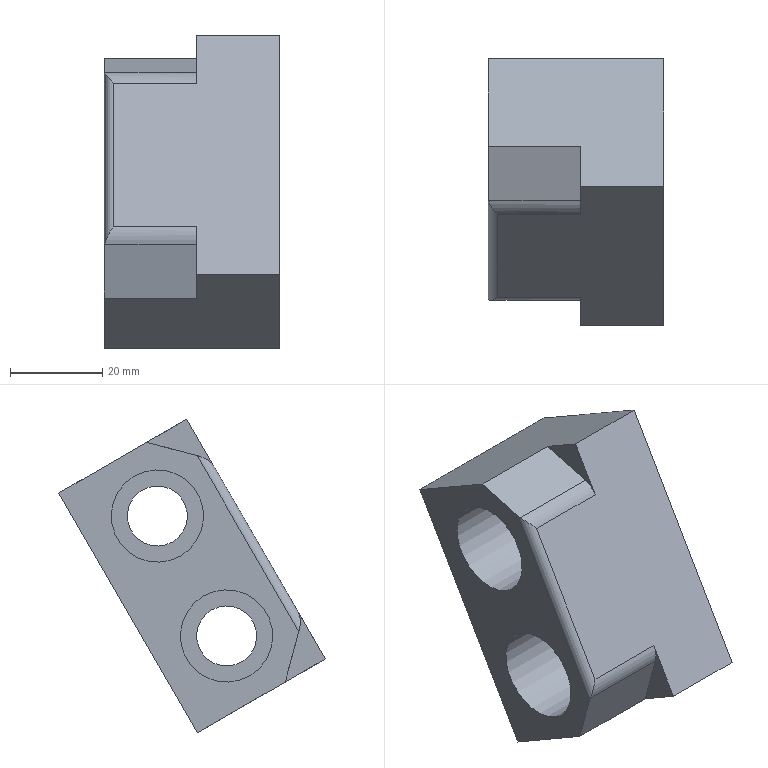Part | NX | features MAIN_BODY 2 | 1 solid | 19 faces | box 38 x 57.713 x 67.962 mm | volume 55374 mm3 | plane 12 | cylinder 7 | commonest cylinder face diameters 10 x2 13 x2 20 x2 4 x1
STEP:
#1=CARTESIAN_POINT('',(-578.,577.963,-16.528));
#2=VERTEX_POINT('',#1);
#3=CARTESIAN_POINT('',(-578.,595.892,14.526));
#4=VERTEX_POINT('',#3);
#5=CARTESIAN_POINT('',(-578.,601.927,24.98));
#6=DIRECTION('',(0.,-0.5,-0.866));
#7=VECTOR('',#6,1000.);
#8=LINE('',#5,#7);
#9=EDGE_CURVE('',#2,#4,#8,.F.);
#10=ORIENTED_EDGE('',*,*,#9,.F.);
#11=CARTESIAN_POINT('',(-560.,577.963,-16.528));
#12=VERTEX_POINT('',#11);
#13=CARTESIAN_POINT('',(-578.,577.963,-16.528));
#14=DIRECTION('',(1.,0.,0.));
#15=VECTOR('',#14,1000.);
#16=LINE('',#13,#15);
#17=EDGE_CURVE('',#12,#2,#16,.F.);
#18=ORIENTED_EDGE('',*,*,#17,.F.);
#19=CARTESIAN_POINT('',(-560.,571.927,-26.982));
#20=VERTEX_POINT('',#19);
#21=CARTESIAN_POINT('',(-560.,601.927,24.98));
#22=DIRECTION('',(0.,-0.5,-0.866));
#23=VECTOR('',#22,1000.);
#24=LINE('',#21,#23);
#25=EDGE_CURVE('',#12,#20,#24,.T.);
#26=ORIENTED_EDGE('',*,*,#25,.T.);
#27=CARTESIAN_POINT('',(-542.,571.927,-26.982));
#28=VERTEX_POINT('',#27);
#29=CARTESIAN_POINT('',(-580.,571.927,-26.982));
#30=DIRECTION('',(1.,0.,0.));
#31=VECTOR('',#30,1000.);
#32=LINE('',#29,#31);
#33=EDGE_CURVE('',#20,#28,#32,.T.);
#34=ORIENTED_EDGE('',*,*,#33,.T.);
#35=CARTESIAN_POINT('',(-542.,601.927,24.98));
#36=VERTEX_POINT('',#35);
#37=CARTESIAN_POINT('',(-542.,601.927,24.98));
#38=DIRECTION('',(0.,-0.5,-0.866));
#39=VECTOR('',#38,1000.);
#40=LINE('',#37,#39);
#41=EDGE_CURVE('',#36,#28,#40,.T.);
#42=ORIENTED_EDGE('',*,*,#41,.F.);
#43=CARTESIAN_POINT('',(-560.,601.927,24.98));
#44=VERTEX_POINT('',#43);
#45=CARTESIAN_POINT('',(-580.,601.927,24.98));
#46=DIRECTION('',(1.,0.,0.));
#47=VECTOR('',#46,1000.);
#48=LINE('',#45,#47);
#49=EDGE_CURVE('',#44,#36,#48,.T.);
#50=ORIENTED_EDGE('',*,*,#49,.F.);
#51=CARTESIAN_POINT('',(-560.,595.892,14.526));
#52=VERTEX_POINT('',#51);
#53=CARTESIAN_POINT('',(-560.,601.927,24.98));
#54=DIRECTION('',(0.,-0.5,-0.866));
#55=VECTOR('',#54,1000.);
#56=LINE('',#53,#55);
#57=EDGE_CURVE('',#44,#52,#56,.T.);
#58=ORIENTED_EDGE('',*,*,#57,.T.);
#59=CARTESIAN_POINT('',(-560.,595.892,14.526));
#60=DIRECTION('',(1.,0.,0.));
#61=VECTOR('',#60,1000.);
#62=LINE('',#59,#61);
#63=EDGE_CURVE('',#4,#52,#62,.T.);
#64=ORIENTED_EDGE('',*,*,#63,.F.);
#65=EDGE_LOOP('',(#10,#18,#26,#34,#42,#50,#58,#64));
#66=FACE_BOUND('',#65,.T.);
#67=CARTESIAN_POINT('',(-580.,601.927,24.98));
#68=DIRECTION('',(0.,0.866,-0.5));
#69=DIRECTION('',(0.,-0.5,-0.866));
#70=AXIS2_PLACEMENT_3D('',#67,#68,#69);
#71=PLANE('',#70);
#72=ADVANCED_FACE('',(#66),#71,.F.);
#73=CARTESIAN_POINT('',(-580.,613.284,12.649));
#74=VERTEX_POINT('',#73);
#75=CARTESIAN_POINT('',(-580.,608.284,3.989));
#76=DIRECTION('',(-1.,0.,0.));
#77=DIRECTION('',(0.,0.5,0.866));
#78=AXIS2_PLACEMENT_3D('',#75,#76,#77);
#79=CIRCLE('',#78,10.);
#80=EDGE_CURVE('',#74,#74,#79,.T.);
#81=ORIENTED_EDGE('',*,*,#80,.F.);
#82=EDGE_LOOP('',(#81));
#83=FACE_BOUND('',#82,.T.);
#84=CARTESIAN_POINT('',(-580.,598.284,-13.331));
#85=VERTEX_POINT('',#84);
#86=CARTESIAN_POINT('',(-580.,593.284,-21.992));
#87=DIRECTION('',(-1.,0.,0.));
#88=DIRECTION('',(0.,0.5,0.866));
#89=AXIS2_PLACEMENT_3D('',#86,#87,#88);
#90=CIRCLE('',#89,10.);
#91=EDGE_CURVE('',#85,#85,#90,.T.);
#92=ORIENTED_EDGE('',*,*,#91,.F.);
#93=EDGE_LOOP('',(#92));
#94=FACE_BOUND('',#93,.T.);
#95=CARTESIAN_POINT('',(-580.,599.659,17.051));
#96=VERTEX_POINT('',#95);
#97=CARTESIAN_POINT('',(-580.,610.588,19.98));
#98=VERTEX_POINT('',#97);
#99=CARTESIAN_POINT('',(-580.,596.927,16.319));
#100=DIRECTION('',(0.,0.9659,0.2588));
#101=VECTOR('',#100,1000.);
#102=LINE('',#99,#101);
#103=EDGE_CURVE('',#96,#98,#102,.T.);
#104=ORIENTED_EDGE('',*,*,#103,.T.);
#105=CARTESIAN_POINT('',(-580.,629.64,8.98));
#106=VERTEX_POINT('',#105);
#107=CARTESIAN_POINT('',(-580.,629.64,8.98));
#108=DIRECTION('',(0.,-0.866,0.5));
#109=VECTOR('',#108,1000.);
#110=LINE('',#107,#109);
#111=EDGE_CURVE('',#106,#98,#110,.T.);
#112=ORIENTED_EDGE('',*,*,#111,.F.);
#113=CARTESIAN_POINT('',(-580.,599.64,-42.982));
#114=VERTEX_POINT('',#113);
#115=CARTESIAN_POINT('',(-580.,599.64,-42.982));
#116=DIRECTION('',(0.,0.5,0.866));
#117=VECTOR('',#116,1000.);
#118=LINE('',#115,#117);
#119=EDGE_CURVE('',#114,#106,#118,.T.);
#120=ORIENTED_EDGE('',*,*,#119,.F.);
#121=CARTESIAN_POINT('',(-580.,580.588,-31.982));
#122=VERTEX_POINT('',#121);
#123=CARTESIAN_POINT('',(-580.,571.927,-26.982));
#124=DIRECTION('',(0.,0.866,-0.5));
#125=VECTOR('',#124,1000.);
#126=LINE('',#123,#125);
#127=EDGE_CURVE('',#122,#114,#126,.T.);
#128=ORIENTED_EDGE('',*,*,#127,.F.);
#129=CARTESIAN_POINT('',(-580.,577.659,-21.054));
#130=VERTEX_POINT('',#129);
#131=CARTESIAN_POINT('',(-580.,580.588,-31.982));
#132=DIRECTION('',(0.,-0.2588,0.9659));
#133=VECTOR('',#132,1000.);
#134=LINE('',#131,#133);
#135=EDGE_CURVE('',#122,#130,#134,.T.);
#136=ORIENTED_EDGE('',*,*,#135,.T.);
#137=CARTESIAN_POINT('',(-580.,573.659,-27.982));
#138=DIRECTION('',(0.,-0.5,-0.866));
#139=VECTOR('',#138,1000.);
#140=LINE('',#137,#139);
#141=EDGE_CURVE('',#96,#130,#140,.T.);
#142=ORIENTED_EDGE('',*,*,#141,.F.);
#143=EDGE_LOOP('',(#104,#112,#120,#128,#136,#142));
#144=FACE_BOUND('',#143,.T.);
#145=CARTESIAN_POINT('',(-580.,599.64,-42.982));
#146=DIRECTION('',(1.,0.,0.));
#147=DIRECTION('',(0.,0.5,0.866));
#148=AXIS2_PLACEMENT_3D('',#145,#146,#147);
#149=PLANE('',#148);
#150=ADVANCED_FACE('',(#83,#94,#144),#149,.F.);
#151=CARTESIAN_POINT('',(-560.,580.588,-31.982));
#152=VERTEX_POINT('',#151);
#153=CARTESIAN_POINT('',(-560.,571.927,-26.982));
#154=DIRECTION('',(0.,0.866,-0.5));
#155=VECTOR('',#154,1000.);
#156=LINE('',#153,#155);
#157=EDGE_CURVE('',#20,#152,#156,.T.);
#158=ORIENTED_EDGE('',*,*,#157,.T.);
#159=CARTESIAN_POINT('',(-580.,580.588,-31.982));
#160=DIRECTION('',(1.,0.,0.));
#161=VECTOR('',#160,1000.);
#162=LINE('',#159,#161);
#163=EDGE_CURVE('',#122,#152,#162,.T.);
#164=ORIENTED_EDGE('',*,*,#163,.F.);
#165=ORIENTED_EDGE('',*,*,#127,.T.);
#166=CARTESIAN_POINT('',(-542.,599.64,-42.982));
#167=VERTEX_POINT('',#166);
#168=CARTESIAN_POINT('',(-580.,599.64,-42.982));
#169=DIRECTION('',(1.,0.,0.));
#170=VECTOR('',#169,1000.);
#171=LINE('',#168,#170);
#172=EDGE_CURVE('',#114,#167,#171,.T.);
#173=ORIENTED_EDGE('',*,*,#172,.T.);
#174=CARTESIAN_POINT('',(-542.,571.927,-26.982));
#175=DIRECTION('',(0.,0.866,-0.5));
#176=VECTOR('',#175,1000.);
#177=LINE('',#174,#176);
#178=EDGE_CURVE('',#28,#167,#177,.T.);
#179=ORIENTED_EDGE('',*,*,#178,.F.);
#180=ORIENTED_EDGE('',*,*,#33,.F.);
#181=EDGE_LOOP('',(#158,#164,#165,#173,#179,#180));
#182=FACE_BOUND('',#181,.T.);
#183=CARTESIAN_POINT('',(-580.,571.927,-26.982));
#184=DIRECTION('',(0.,0.5,0.866));
#185=DIRECTION('',(-1.,0.,0.));
#186=AXIS2_PLACEMENT_3D('',#183,#184,#185);
#187=PLANE('',#186);
#188=ADVANCED_FACE('',(#182),#187,.F.);
#189=CARTESIAN_POINT('',(-560.,610.588,19.98));
#190=VERTEX_POINT('',#189);
#191=CARTESIAN_POINT('',(-560.,629.64,8.98));
#192=DIRECTION('',(0.,-0.866,0.5));
#193=VECTOR('',#192,1000.);
#194=LINE('',#191,#193);
#195=EDGE_CURVE('',#190,#44,#194,.T.);
#196=ORIENTED_EDGE('',*,*,#195,.T.);
#197=ORIENTED_EDGE('',*,*,#49,.T.);
#198=CARTESIAN_POINT('',(-542.,629.64,8.98));
#199=VERTEX_POINT('',#198);
#200=CARTESIAN_POINT('',(-542.,629.64,8.98));
#201=DIRECTION('',(0.,-0.866,0.5));
#202=VECTOR('',#201,1000.);
#203=LINE('',#200,#202);
#204=EDGE_CURVE('',#199,#36,#203,.T.);
#205=ORIENTED_EDGE('',*,*,#204,.F.);
#206=CARTESIAN_POINT('',(-580.,629.64,8.98));
#207=DIRECTION('',(1.,0.,0.));
#208=VECTOR('',#207,1000.);
#209=LINE('',#206,#208);
#210=EDGE_CURVE('',#106,#199,#209,.T.);
#211=ORIENTED_EDGE('',*,*,#210,.F.);
#212=ORIENTED_EDGE('',*,*,#111,.T.);
#213=CARTESIAN_POINT('',(-580.,610.588,19.98));
#214=DIRECTION('',(1.,0.,0.));
#215=VECTOR('',#214,1000.);
#216=LINE('',#213,#215);
#217=EDGE_CURVE('',#98,#190,#216,.T.);
#218=ORIENTED_EDGE('',*,*,#217,.T.);
#219=EDGE_LOOP('',(#196,#197,#205,#211,#212,#218));
#220=FACE_BOUND('',#219,.T.);
#221=CARTESIAN_POINT('',(-580.,629.64,8.98));
#222=DIRECTION('',(0.,-0.5,-0.866));
#223=DIRECTION('',(0.,-0.866,0.5));
#224=AXIS2_PLACEMENT_3D('',#221,#222,#223);
#225=PLANE('',#224);
#226=ADVANCED_FACE('',(#220),#225,.F.);
#227=CARTESIAN_POINT('',(-542.,599.64,-42.982));
#228=DIRECTION('',(0.,0.5,0.866));
#229=VECTOR('',#228,1000.);
#230=LINE('',#227,#229);
#231=EDGE_CURVE('',#167,#199,#230,.T.);
#232=ORIENTED_EDGE('',*,*,#231,.F.);
#233=ORIENTED_EDGE('',*,*,#172,.F.);
#234=ORIENTED_EDGE('',*,*,#119,.T.);
#235=ORIENTED_EDGE('',*,*,#210,.T.);
#236=EDGE_LOOP('',(#232,#233,#234,#235));
#237=FACE_BOUND('',#236,.T.);
#238=CARTESIAN_POINT('',(-580.,599.64,-42.982));
#239=DIRECTION('',(0.,-0.866,0.5));
#240=DIRECTION('',(-1.,0.,0.));
#241=AXIS2_PLACEMENT_3D('',#238,#239,#240);
#242=PLANE('',#241);
#243=ADVANCED_FACE('',(#237),#242,.F.);
#244=CARTESIAN_POINT('',(-565.,611.534,9.618));
#245=VERTEX_POINT('',#244);
#246=CARTESIAN_POINT('',(-565.,608.284,3.989));
#247=DIRECTION('',(-1.,0.,0.));
#248=DIRECTION('',(0.,0.5,0.866));
#249=AXIS2_PLACEMENT_3D('',#246,#247,#248);
#250=CIRCLE('',#249,6.5);
#251=EDGE_CURVE('',#245,#245,#250,.F.);
#252=ORIENTED_EDGE('',*,*,#251,.F.);
#253=EDGE_LOOP('',(#252));
#254=FACE_BOUND('',#253,.T.);
#255=CARTESIAN_POINT('',(-542.,611.534,9.618));
#256=VERTEX_POINT('',#255);
#257=CARTESIAN_POINT('',(-542.,608.284,3.989));
#258=DIRECTION('',(-1.,0.,0.));
#259=DIRECTION('',(0.,0.5,0.866));
#260=AXIS2_PLACEMENT_3D('',#257,#258,#259);
#261=CIRCLE('',#260,6.5);
#262=EDGE_CURVE('',#256,#256,#261,.T.);
#263=ORIENTED_EDGE('',*,*,#262,.F.);
#264=EDGE_LOOP('',(#263));
#265=FACE_BOUND('',#264,.T.);
#266=CARTESIAN_POINT('',(-580.,608.284,3.989));
#267=DIRECTION('',(1.,0.,0.));
#268=DIRECTION('',(0.,0.5,0.866));
#269=AXIS2_PLACEMENT_3D('',#266,#267,#268);
#270=CYLINDRICAL_SURFACE('',#269,6.5);
#271=ADVANCED_FACE('',(#254,#265),#270,.F.);
#272=CARTESIAN_POINT('',(-565.,596.534,-16.362));
#273=VERTEX_POINT('',#272);
#274=CARTESIAN_POINT('',(-565.,593.284,-21.992));
#275=DIRECTION('',(-1.,0.,0.));
#276=DIRECTION('',(0.,0.5,0.866));
#277=AXIS2_PLACEMENT_3D('',#274,#275,#276);
#278=CIRCLE('',#277,6.5);
#279=EDGE_CURVE('',#273,#273,#278,.F.);
#280=ORIENTED_EDGE('',*,*,#279,.F.);
#281=EDGE_LOOP('',(#280));
#282=FACE_BOUND('',#281,.T.);
#283=CARTESIAN_POINT('',(-542.,596.534,-16.362));
#284=VERTEX_POINT('',#283);
#285=CARTESIAN_POINT('',(-542.,593.284,-21.992));
#286=DIRECTION('',(-1.,0.,0.));
#287=DIRECTION('',(0.,0.5,0.866));
#288=AXIS2_PLACEMENT_3D('',#285,#286,#287);
#289=CIRCLE('',#288,6.5);
#290=EDGE_CURVE('',#284,#284,#289,.T.);
#291=ORIENTED_EDGE('',*,*,#290,.F.);
#292=EDGE_LOOP('',(#291));
#293=FACE_BOUND('',#292,.T.);
#294=CARTESIAN_POINT('',(-580.,593.284,-21.992));
#295=DIRECTION('',(1.,0.,0.));
#296=DIRECTION('',(0.,0.5,0.866));
#297=AXIS2_PLACEMENT_3D('',#294,#295,#296);
#298=CYLINDRICAL_SURFACE('',#297,6.5);
#299=ADVANCED_FACE('',(#282,#293),#298,.F.);
#300=ORIENTED_EDGE('',*,*,#262,.T.);
#301=EDGE_LOOP('',(#300));
#302=FACE_BOUND('',#301,.T.);
#303=ORIENTED_EDGE('',*,*,#231,.T.);
#304=ORIENTED_EDGE('',*,*,#204,.T.);
#305=ORIENTED_EDGE('',*,*,#41,.T.);
#306=ORIENTED_EDGE('',*,*,#178,.T.);
#307=EDGE_LOOP('',(#303,#304,#305,#306));
#308=FACE_BOUND('',#307,.T.);
#309=ORIENTED_EDGE('',*,*,#290,.T.);
#310=EDGE_LOOP('',(#309));
#311=FACE_BOUND('',#310,.T.);
#312=CARTESIAN_POINT('',(-542.,599.64,-42.982));
#313=DIRECTION('',(1.,0.,0.));
#314=DIRECTION('',(0.,0.5,0.866));
#315=AXIS2_PLACEMENT_3D('',#312,#313,#314);
#316=PLANE('',#315);
#317=ADVANCED_FACE('',(#302,#308,#311),#316,.T.);
#318=CARTESIAN_POINT('',(-565.,598.284,-13.331));
#319=VERTEX_POINT('',#318);
#320=CARTESIAN_POINT('',(-565.,593.284,-21.992));
#321=DIRECTION('',(-1.,0.,0.));
#322=DIRECTION('',(0.,0.5,0.866));
#323=AXIS2_PLACEMENT_3D('',#320,#321,#322);
#324=CIRCLE('',#323,10.);
#325=EDGE_CURVE('',#319,#319,#324,.T.);
#326=ORIENTED_EDGE('',*,*,#325,.T.);
#327=EDGE_LOOP('',(#326));
#328=FACE_BOUND('',#327,.T.);
#329=ORIENTED_EDGE('',*,*,#279,.T.);
#330=EDGE_LOOP('',(#329));
#331=FACE_BOUND('',#330,.T.);
#332=CARTESIAN_POINT('',(-565.,593.284,-21.992));
#333=DIRECTION('',(1.,0.,0.));
#334=DIRECTION('',(0.,0.5,0.866));
#335=AXIS2_PLACEMENT_3D('',#332,#333,#334);
#336=PLANE('',#335);
#337=ADVANCED_FACE('',(#328,#331),#336,.F.);
#338=ORIENTED_EDGE('',*,*,#91,.T.);
#339=EDGE_LOOP('',(#338));
#340=FACE_BOUND('',#339,.T.);
#341=ORIENTED_EDGE('',*,*,#325,.F.);
#342=EDGE_LOOP('',(#341));
#343=FACE_BOUND('',#342,.T.);
#344=CARTESIAN_POINT('',(-580.,593.284,-21.992));
#345=DIRECTION('',(1.,0.,0.));
#346=DIRECTION('',(0.,0.5,0.866));
#347=AXIS2_PLACEMENT_3D('',#344,#345,#346);
#348=CYLINDRICAL_SURFACE('',#347,10.);
#349=ADVANCED_FACE('',(#340,#343),#348,.F.);
#350=CARTESIAN_POINT('',(-565.,613.284,12.649));
#351=VERTEX_POINT('',#350);
#352=CARTESIAN_POINT('',(-565.,608.284,3.989));
#353=DIRECTION('',(-1.,0.,0.));
#354=DIRECTION('',(0.,0.5,0.866));
#355=AXIS2_PLACEMENT_3D('',#352,#353,#354);
#356=CIRCLE('',#355,10.);
#357=EDGE_CURVE('',#351,#351,#356,.T.);
#358=ORIENTED_EDGE('',*,*,#357,.T.);
#359=EDGE_LOOP('',(#358));
#360=FACE_BOUND('',#359,.T.);
#361=ORIENTED_EDGE('',*,*,#251,.T.);
#362=EDGE_LOOP('',(#361));
#363=FACE_BOUND('',#362,.T.);
#364=CARTESIAN_POINT('',(-565.,608.284,3.989));
#365=DIRECTION('',(1.,0.,0.));
#366=DIRECTION('',(0.,0.5,0.866));
#367=AXIS2_PLACEMENT_3D('',#364,#365,#366);
#368=PLANE('',#367);
#369=ADVANCED_FACE('',(#360,#363),#368,.F.);
#370=ORIENTED_EDGE('',*,*,#80,.T.);
#371=EDGE_LOOP('',(#370));
#372=FACE_BOUND('',#371,.T.);
#373=ORIENTED_EDGE('',*,*,#357,.F.);
#374=EDGE_LOOP('',(#373));
#375=FACE_BOUND('',#374,.T.);
#376=CARTESIAN_POINT('',(-580.,608.284,3.989));
#377=DIRECTION('',(1.,0.,0.));
#378=DIRECTION('',(0.,0.5,0.866));
#379=AXIS2_PLACEMENT_3D('',#376,#377,#378);
#380=CYLINDRICAL_SURFACE('',#379,10.);
#381=ADVANCED_FACE('',(#372,#375),#380,.F.);
#382=ORIENTED_EDGE('',*,*,#195,.F.);
#383=CARTESIAN_POINT('',(-560.,598.928,16.855));
#384=VERTEX_POINT('',#383);
#385=CARTESIAN_POINT('',(-560.,596.927,16.319));
#386=DIRECTION('',(0.,0.9659,0.2588));
#387=VECTOR('',#386,1000.);
#388=LINE('',#385,#387);
#389=EDGE_CURVE('',#384,#190,#388,.T.);
#390=ORIENTED_EDGE('',*,*,#389,.F.);
#391=CARTESIAN_POINT('',(-560.,600.222,12.026));
#392=DIRECTION('',(1.,0.,0.));
#393=DIRECTION('',(0.,-0.5,-0.866));
#394=AXIS2_PLACEMENT_3D('',#391,#392,#393);
#395=CIRCLE('',#394,5.);
#396=EDGE_CURVE('',#52,#384,#395,.F.);
#397=ORIENTED_EDGE('',*,*,#396,.F.);
#398=ORIENTED_EDGE('',*,*,#57,.F.);
#399=EDGE_LOOP('',(#382,#390,#397,#398));
#400=FACE_BOUND('',#399,.T.);
#401=CARTESIAN_POINT('',(-560.,596.927,16.319));
#402=DIRECTION('',(-1.,0.,0.));
#403=DIRECTION('',(0.,0.9659,0.2588));
#404=AXIS2_PLACEMENT_3D('',#401,#402,#403);
#405=PLANE('',#404);
#406=ADVANCED_FACE('',(#400),#405,.T.);
#407=ORIENTED_EDGE('',*,*,#389,.T.);
#408=ORIENTED_EDGE('',*,*,#217,.F.);
#409=ORIENTED_EDGE('',*,*,#103,.F.);
#410=CARTESIAN_POINT('',(-579.927,598.928,16.855));
#411=VERTEX_POINT('',#410);
#412=CARTESIAN_POINT('',(-578.,599.659,17.051));
#413=DIRECTION('',(0.,0.2588,-0.9659));
#414=DIRECTION('',(0.,-0.9659,-0.2588));
#415=AXIS2_PLACEMENT_3D('',#412,#413,#414);
#416=ELLIPSE('',#415,2.828,2.);
#417=EDGE_CURVE('',#411,#96,#416,.T.);
#418=ORIENTED_EDGE('',*,*,#417,.F.);
#419=CARTESIAN_POINT('',(-578.,598.928,16.855));
#420=DIRECTION('',(1.,0.,0.));
#421=VECTOR('',#420,1000.);
#422=LINE('',#419,#421);
#423=EDGE_CURVE('',#384,#411,#422,.F.);
#424=ORIENTED_EDGE('',*,*,#423,.F.);
#425=EDGE_LOOP('',(#407,#408,#409,#418,#424));
#426=FACE_BOUND('',#425,.T.);
#427=CARTESIAN_POINT('',(-580.,596.927,16.319));
#428=DIRECTION('',(0.,-0.2588,0.9659));
#429=DIRECTION('',(0.,0.9659,0.2588));
#430=AXIS2_PLACEMENT_3D('',#427,#428,#429);
#431=PLANE('',#430);
#432=ADVANCED_FACE('',(#426),#431,.T.);
#433=ORIENTED_EDGE('',*,*,#25,.F.);
#434=CARTESIAN_POINT('',(-560.,577.463,-20.322));
#435=VERTEX_POINT('',#434);
#436=CARTESIAN_POINT('',(-560.,582.293,-19.028));
#437=DIRECTION('',(1.,0.,0.));
#438=DIRECTION('',(0.,-0.5,-0.866));
#439=AXIS2_PLACEMENT_3D('',#436,#437,#438);
#440=CIRCLE('',#439,5.);
#441=EDGE_CURVE('',#435,#12,#440,.F.);
#442=ORIENTED_EDGE('',*,*,#441,.F.);
#443=CARTESIAN_POINT('',(-560.,580.588,-31.982));
#444=DIRECTION('',(0.,-0.2588,0.9659));
#445=VECTOR('',#444,1000.);
#446=LINE('',#443,#445);
#447=EDGE_CURVE('',#152,#435,#446,.T.);
#448=ORIENTED_EDGE('',*,*,#447,.F.);
#449=ORIENTED_EDGE('',*,*,#157,.F.);
#450=EDGE_LOOP('',(#433,#442,#448,#449));
#451=FACE_BOUND('',#450,.T.);
#452=CARTESIAN_POINT('',(-560.,580.588,-31.982));
#453=DIRECTION('',(-1.,0.,0.));
#454=DIRECTION('',(0.,-0.2588,0.9659));
#455=AXIS2_PLACEMENT_3D('',#452,#453,#454);
#456=PLANE('',#455);
#457=ADVANCED_FACE('',(#451),#456,.T.);
#458=CARTESIAN_POINT('',(-579.927,577.463,-20.322));
#459=VERTEX_POINT('',#458);
#460=CARTESIAN_POINT('',(-578.,577.659,-21.054));
#461=DIRECTION('',(0.,0.9659,0.2588));
#462=DIRECTION('',(0.,0.2588,-0.9659));
#463=AXIS2_PLACEMENT_3D('',#460,#461,#462);
#464=ELLIPSE('',#463,2.828,2.);
#465=EDGE_CURVE('',#130,#459,#464,.T.);
#466=ORIENTED_EDGE('',*,*,#465,.F.);
#467=ORIENTED_EDGE('',*,*,#135,.F.);
#468=ORIENTED_EDGE('',*,*,#163,.T.);
#469=ORIENTED_EDGE('',*,*,#447,.T.);
#470=CARTESIAN_POINT('',(-560.,577.463,-20.322));
#471=DIRECTION('',(1.,0.,0.));
#472=VECTOR('',#471,1000.);
#473=LINE('',#470,#472);
#474=EDGE_CURVE('',#459,#435,#473,.T.);
#475=ORIENTED_EDGE('',*,*,#474,.F.);
#476=EDGE_LOOP('',(#466,#467,#468,#469,#475));
#477=FACE_BOUND('',#476,.T.);
#478=CARTESIAN_POINT('',(-580.,580.588,-31.982));
#479=DIRECTION('',(0.,-0.9659,-0.2588));
#480=DIRECTION('',(0.,-0.2588,0.9659));
#481=AXIS2_PLACEMENT_3D('',#478,#479,#480);
#482=PLANE('',#481);
#483=ADVANCED_FACE('',(#477),#482,.T.);
#484=ORIENTED_EDGE('',*,*,#417,.T.);
#485=ORIENTED_EDGE('',*,*,#141,.T.);
#486=ORIENTED_EDGE('',*,*,#465,.T.);
#487=CARTESIAN_POINT('',(-579.927,577.463,-20.322));
#488=CARTESIAN_POINT('',(-579.641,577.087,-18.917));
#489=CARTESIAN_POINT('',(-578.781,577.345,-17.598));
#490=CARTESIAN_POINT('',(-578.,577.963,-16.528));
#491=B_SPLINE_CURVE_WITH_KNOTS('',3,(#487,#488,#489,#490),.UNSPECIFIED.,.F.,.F.,(4,4),(0.,0.004383),.UNSPECIFIED.);
#492=EDGE_CURVE('',#2,#459,#491,.F.);
#493=ORIENTED_EDGE('',*,*,#492,.F.);
#494=ORIENTED_EDGE('',*,*,#9,.T.);
#495=CARTESIAN_POINT('',(-579.927,598.928,16.855));
#496=CARTESIAN_POINT('',(-579.641,597.522,16.479));
#497=CARTESIAN_POINT('',(-578.781,596.509,15.595));
#498=CARTESIAN_POINT('',(-578.,595.892,14.526));
#499=B_SPLINE_CURVE_WITH_KNOTS('',3,(#495,#496,#497,#498),.UNSPECIFIED.,.F.,.F.,(4,4),(0.,0.004383),.UNSPECIFIED.);
#500=EDGE_CURVE('',#411,#4,#499,.T.);
#501=ORIENTED_EDGE('',*,*,#500,.F.);
#502=EDGE_LOOP('',(#484,#485,#486,#493,#494,#501));
#503=FACE_BOUND('',#502,.T.);
#504=CARTESIAN_POINT('',(-578.,573.659,-27.982));
#505=DIRECTION('',(0.,-0.5,-0.866));
#506=DIRECTION('',(0.,-0.866,0.5));
#507=AXIS2_PLACEMENT_3D('',#504,#505,#506);
#508=CYLINDRICAL_SURFACE('',#507,2.);
#509=ADVANCED_FACE('',(#503),#508,.T.);
#510=ORIENTED_EDGE('',*,*,#500,.T.);
#511=ORIENTED_EDGE('',*,*,#63,.T.);
#512=ORIENTED_EDGE('',*,*,#396,.T.);
#513=ORIENTED_EDGE('',*,*,#423,.T.);
#514=EDGE_LOOP('',(#510,#511,#512,#513));
#515=FACE_BOUND('',#514,.T.);
#516=CARTESIAN_POINT('',(-580.,600.222,12.026));
#517=DIRECTION('',(-1.,0.,0.));
#518=DIRECTION('',(0.,-0.5,-0.866));
#519=AXIS2_PLACEMENT_3D('',#516,#517,#518);
#520=CYLINDRICAL_SURFACE('',#519,5.);
#521=ADVANCED_FACE('',(#515),#520,.T.);
#522=ORIENTED_EDGE('',*,*,#492,.T.);
#523=ORIENTED_EDGE('',*,*,#474,.T.);
#524=ORIENTED_EDGE('',*,*,#441,.T.);
#525=ORIENTED_EDGE('',*,*,#17,.T.);
#526=EDGE_LOOP('',(#522,#523,#524,#525));
#527=FACE_BOUND('',#526,.T.);
#528=CARTESIAN_POINT('',(-580.,582.293,-19.028));
#529=DIRECTION('',(-1.,0.,0.));
#530=DIRECTION('',(0.,-0.5,-0.866));
#531=AXIS2_PLACEMENT_3D('',#528,#529,#530);
#532=CYLINDRICAL_SURFACE('',#531,5.);
#533=ADVANCED_FACE('',(#527),#532,.T.);
#534=CLOSED_SHELL('',(#72,#150,#188,#226,#243,#271,#299,#317,#337,#349,#369,#381,#406,#432,#457,#483,#509,#521,#533));
#535=MANIFOLD_SOLID_BREP('',#534);
#536=(LENGTH_UNIT()NAMED_UNIT(*)SI_UNIT(.MILLI.,.METRE.));
#537=UNCERTAINTY_MEASURE_WITH_UNIT(LENGTH_MEASURE(0.0508),#536,'','');
#538=(NAMED_UNIT(*)PLANE_ANGLE_UNIT()SI_UNIT($,.RADIAN.));
#539=(NAMED_UNIT(*)SI_UNIT($,.STERADIAN.)SOLID_ANGLE_UNIT());
#540=(GEOMETRIC_REPRESENTATION_CONTEXT(3)GLOBAL_UNCERTAINTY_ASSIGNED_CONTEXT((#537))GLOBAL_UNIT_ASSIGNED_CONTEXT((#536,#538,#539))REPRESENTATION_CONTEXT('',''));
#541=ADVANCED_BREP_SHAPE_REPRESENTATION('',(#535),#540);